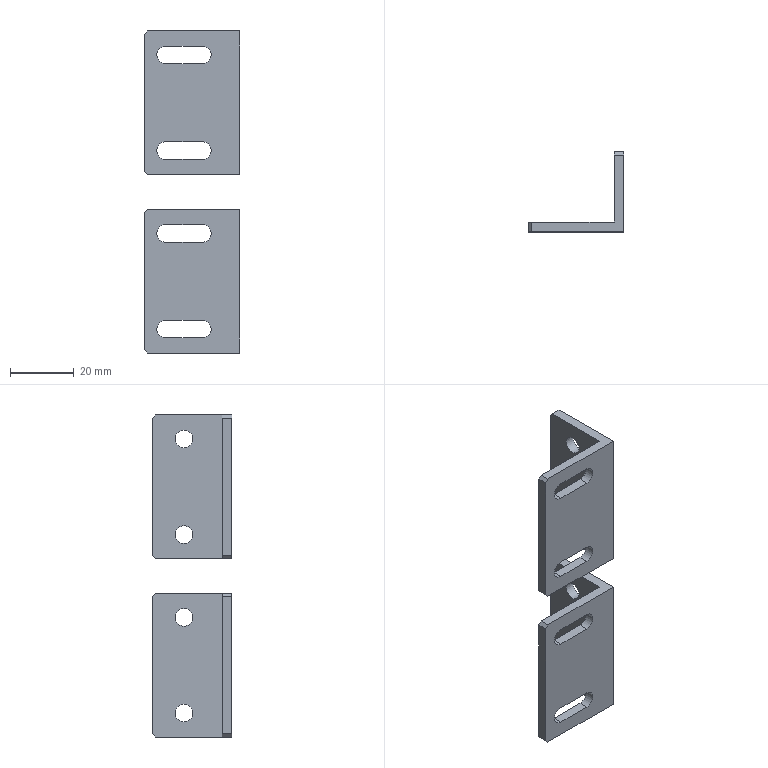CAM job | NX | 3+2 milling | part box 30 x 25 x 101 mm | stock box 35 x 30 x 106 mm
Operations:
program,operation,operation_type,tool,method,geometry_group,spindle_rpm,surface_speed,feed_per_tooth,feed_cut,feed_plunge,cut_length_mm,path_length_mm,cut_time_min,machine_time_min
A,顶面,FaceMilling,D80R0.8飞刀,侧刃精光-切深K-步距G,W-A,4000.0,1005.31,0.125,1000.0,100.0,195.0,231.0,0.195,0.1986
A,动态开粗D10_COPY,CavityMilling,D8,动态开粗-切深K-步距K,W-A,8000.0,251.32,0.25,4000.0,100.0,15535.841,16643.91,3.884,3.995
A,通腰槽粗_1,VolumeBased25DMillingOperation,D4,METHOD,W-A,6000.0,75.398,0.1,1200.0,100.0,1956.123,2387.436,1.63,1.673
A,腰槽精_1,VolumeBased25DMillingOperation,D4-J,METHOD,W-A,6000.0,113.0,0.0667,800.0,100.0,119.763,566.796,0.1497,0.1944
A,仅选体,SurfaceContour,D6倒角刀,METHOD,W-A,8000.0,150.796,0.1875,3000.0,100.0,671.028,1403.439,0.2237,0.2969
A,底壁铣倒角_COPY,VolumeBased25DMillingOperation,D6倒角刀,爬面_倒角-切深0-步距G,W-A,6500.0,122.519,0.1154,1500.0,100.0,47.202,331.761,0.0315,0.0599
A,底壁铣精光底面-中_COPY,VolumeBased25DMillingOperation,D10-J,精光步距切深关,W-A,7000.0,175.0,0.0536,1500.0,100.0,692.799,754.799,0.4619,0.4681
A,等高精光-中_COPY,ZLevelMilling,D10-J,侧刃精光-切深K-步距G,W-A,8000.0,251.32,0.0625,1000.0,100.0,1053.109,1673.758,1.053,1.115